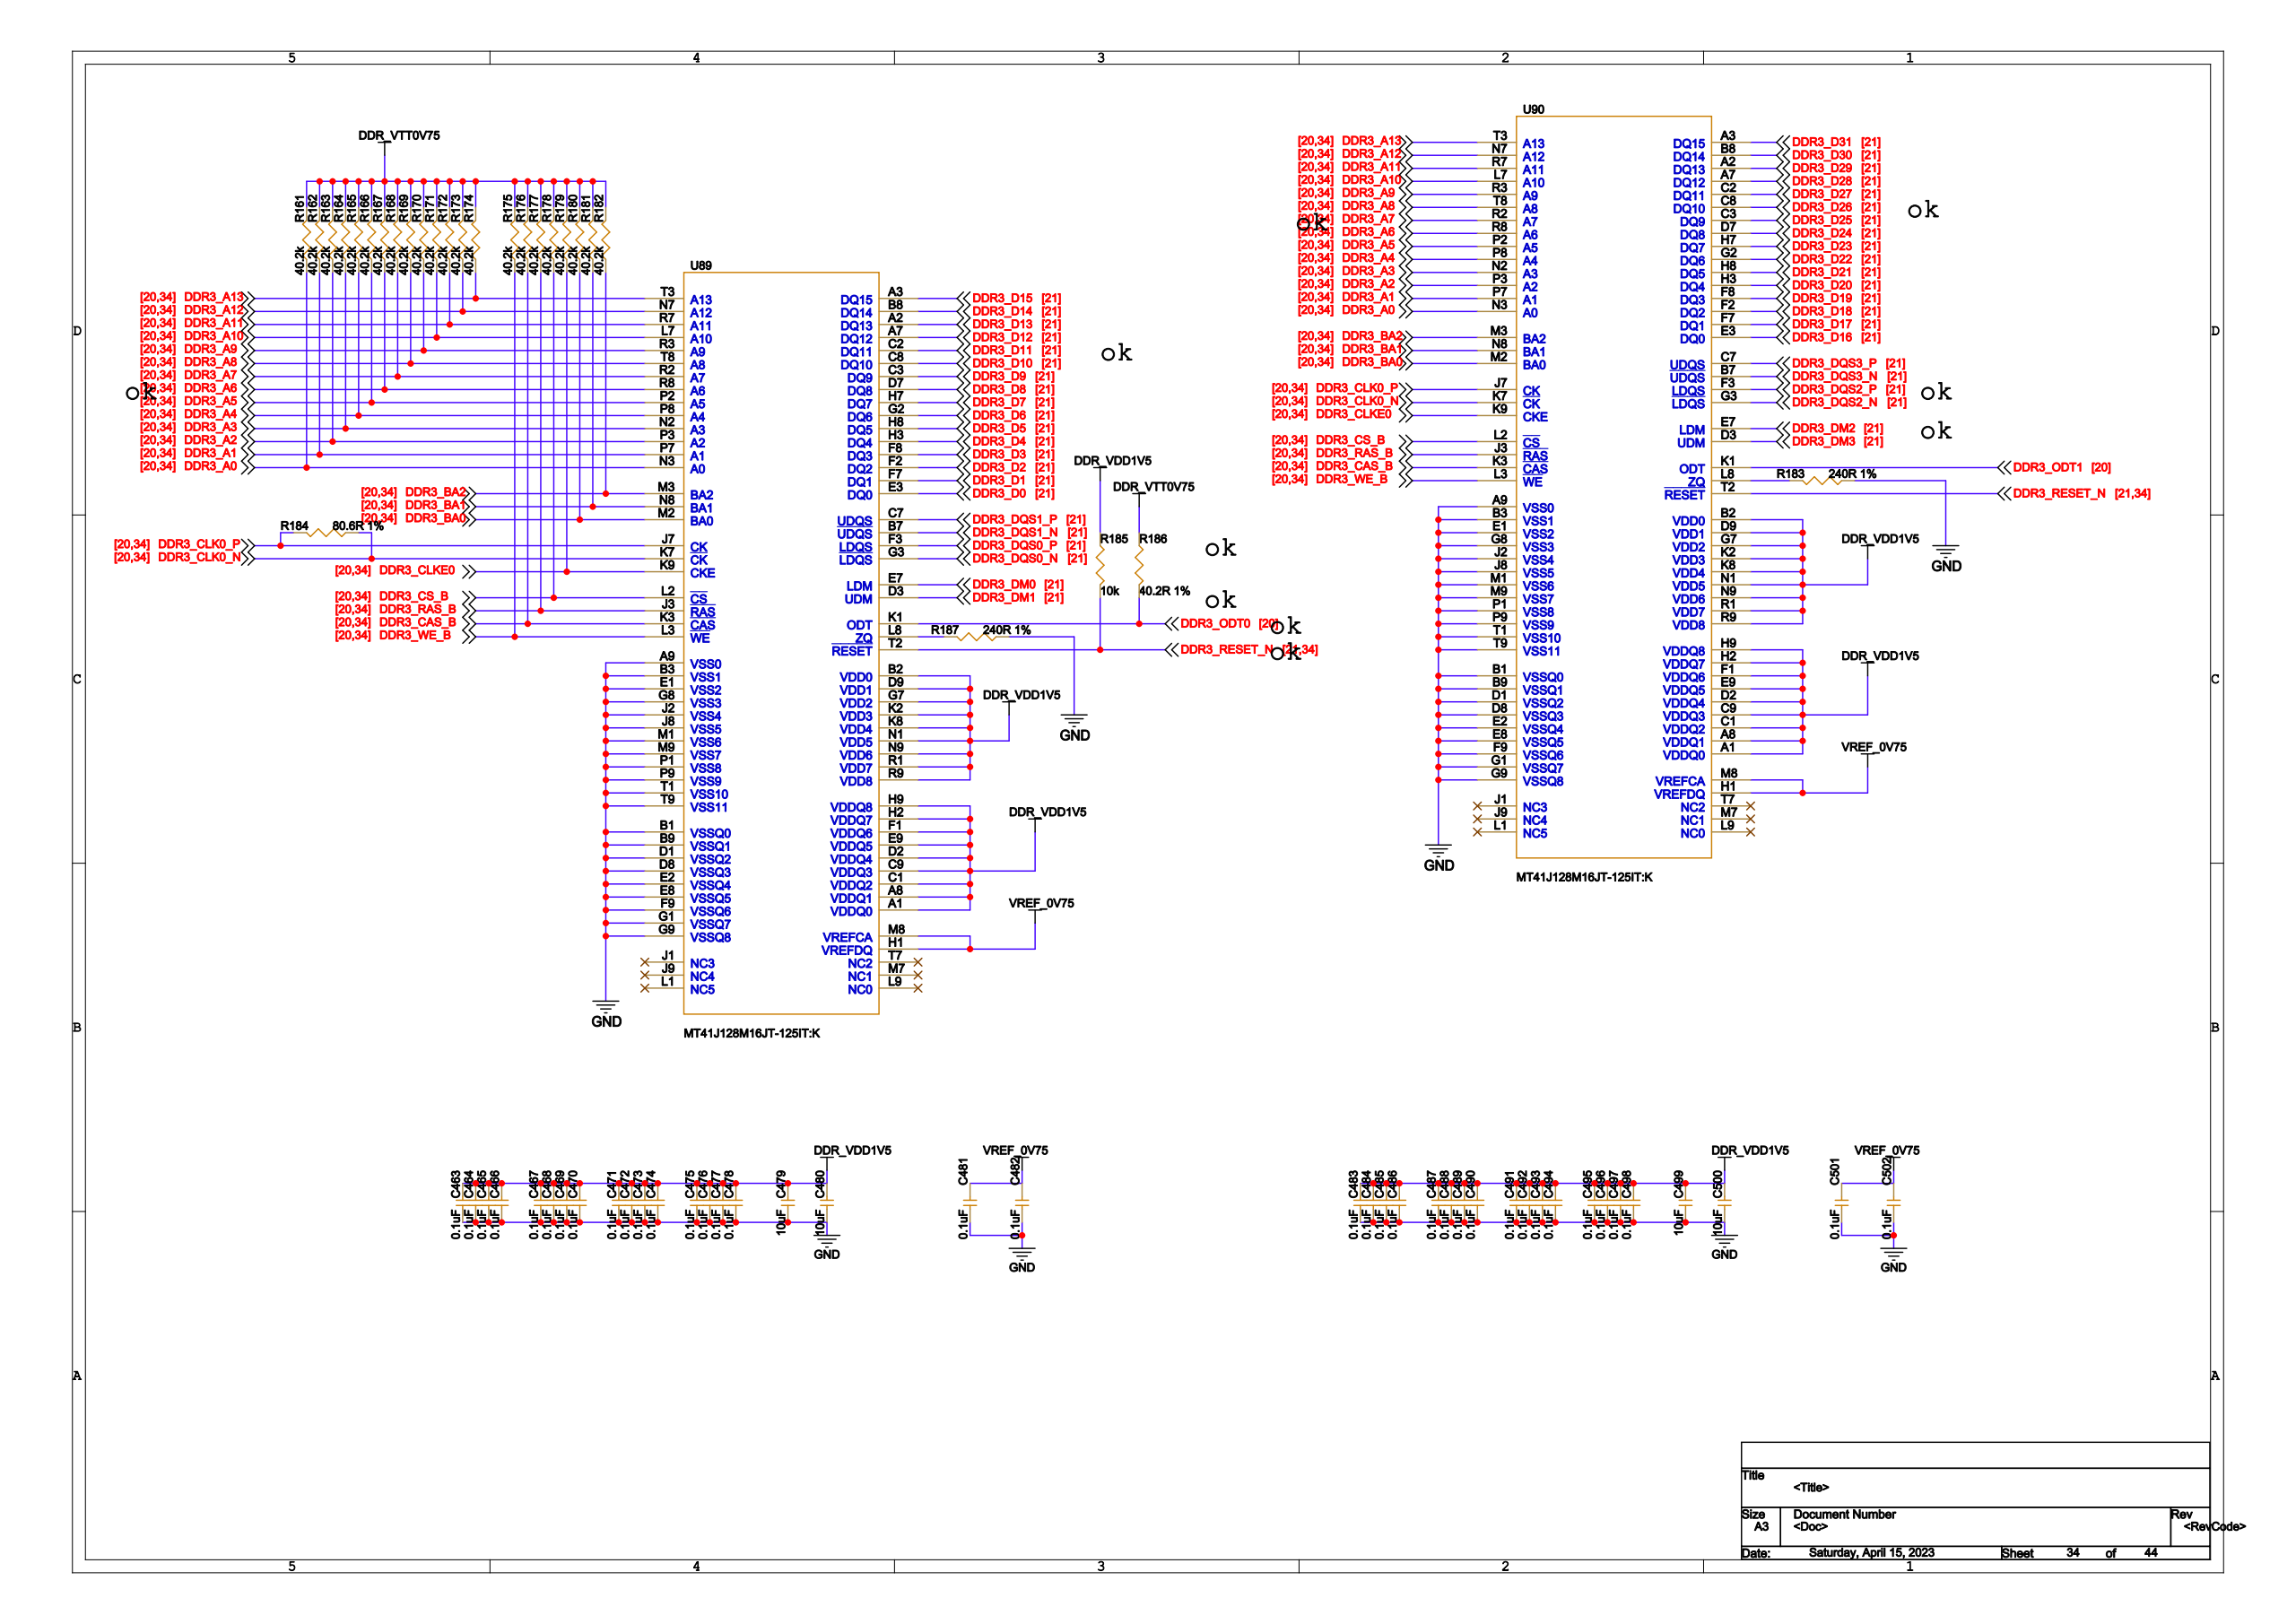Circuit board | Cadence Allegro | 1034 parts | 912 nets | one sheet of the schematic
Parts on this sheet (reference | value | footprint):
C463 | 0.1uF | C0402
C464 | 0.1uF | C0402
C465 | 0.1uF | C0402
C466 | 0.1uF | C0402
C467 | 0.1uF | C0402
C468 | 0.1uF | C0402
C469 | 0.1uF | C0402
C470 | 0.1uF | C0402
C471 | 0.1uF | C0402
C472 | 0.1uF | C0402
C473 | 0.1uF | C0402
C474 | 0.1uF | C0402
C475 | 0.1uF | C0402
C476 | 0.1uF | C0402
C477 | 0.1uF | C0402
C478 | 0.1uF | C0402
C479 | 10uF | C0402
C480 | 10uF | C0402
C481 | 0.1uF | C0402
C482 | 0.1uF | C0402
C483 | 0.1uF | C0402
C484 | 0.1uF | C0402
C485 | 0.1uF | C0402
C486 | 0.1uF | C0402
C487 | 0.1uF | C0402
C488 | 0.1uF | C0402
C489 | 0.1uF | C0402
C490 | 0.1uF | C0402
C491 | 0.1uF | C0402
C492 | 0.1uF | C0402
C493 | 0.1uF | C0402
C494 | 0.1uF | C0402
C495 | 0.1uF | C0402
C496 | 0.1uF | C0402
C497 | 0.1uF | C0402
C498 | 0.1uF | C0402
C499 | 10uF | C0402
C500 | 10uF | C0402
C501 | 0.1uF | C0402
C502 | 0.1uF | C0402
P1 | TSW-120-07-G-D | TSW_2MM54_DR
P3 | TSW-120-07-G-D | TSW_2MM54_DR
R161 | 40.2k | R0402
R162 | 40.2k | R0402
R163 | 40.2k | R0402
R164 | 40.2k | R0402
R165 | 40.2k | R0402
R166 | 40.2k | R0402
R167 | 40.2k | R0402
R168 | 40.2k | R0402
R169 | 40.2k | R0402
R170 | 40.2k | R0402
R171 | 40.2k | R0402
R172 | 40.2k | R0402
R173 | 40.2k | R0402
R174 | 40.2k | R0402
R175 | 40.2k | R0402
R176 | 40.2k | R0402
R177 | 40.2k | R0402
R178 | 40.2k | R0402
R179 | 40.2k | R0402
R180 | 40.2k | R0402
R181 | 40.2k | R0402
R182 | 40.2k | R0402
R183 | 240R 1% | R0402
R184 | 80.6R 1% | R0402
R185 | 10k | R0402
R186 | 40.2R 1% | R0402
R187 | 240R 1% | R0402
U89 | MT41J128M16JT-125IT:K | FBGA_96BALL
U90 | MT41J128M16JT-125IT:K | FBGA_96BALL
Nets of these parts (net: part-pin ...):
GND: C463-1 C464-1 C465-1 C466-1 C467-1 C468-1 C469-1 C470-1 C471-1 C472-1 C473-1 C474-1 C475-1 C476-1 C477-1 C478-1 C479-1 C480-1 C481-1 C482-1 C483-1 C484-1 C485-1 C486-1 C487-1 C488-1 C489-1 C490-1 C491-1 C492-1 C493-1 C494-1 C495-1 C496-1 C497-1 C498-1 C499-1 C500-1 C501-1 C502-1 R183-1 R187-1 P1-1 P1-2 P1-3 P1-4 P1-15 P1-34 P3-1 P3-2 P3-3 P3-15 U89-A9 U89-B1 U89-B3 U89-B9 U89-D1 U89-D8 U89-E1 U89-E2 U89-E8 U89-F9 U89-G1 U89-G8 U89-G9 U89-J2 U89-J8 U89-M1 U89-M9 U89-P1 U89-P9 U89-T1 U89-T9 U90-A9 U90-B1 U90-B3 U90-B9 U90-D1 U90-D8 U90-E1 U90-E2 U90-E8 U90-F9 U90-G1 U90-G8 U90-G9 U90-J2 U90-J8 U90-M1 U90-M9 U90-P1 U90-P9 U90-T1 U90-T9
VREF_0V75: C481-2 C482-2 C501-2 C502-2 U89-H1 U89-M8 U90-H1 U90-M8
DDR3_CLK0_N: R184-1 U89-K7 U90-K7
DDR3_CLK0_P: R184-2 U89-J7 U90-J7
DDR_VTT0V75: R161-2 R162-2 R163-2 R164-2 R165-2 R166-2 R167-2 R168-2 R169-2 R170-2 R171-2 R172-2 R173-2 R174-2 R175-2 R176-2 R177-2 R178-2 R179-2 R180-2 R181-2 R182-2 R186-1
DDR3_ODT0: R186-2 U89-K1
DDR_VDD1V5: C463-2 C464-2 C465-2 C466-2 C467-2 C468-2 C469-2 C470-2 C471-2 C472-2 C473-2 C474-2 C475-2 C476-2 C477-2 C478-2 C479-2 C480-2 C483-2 C484-2 C485-2 C486-2 C487-2 C488-2 C489-2 C490-2 C491-2 C492-2 C493-2 C494-2 C495-2 C496-2 C497-2 C498-2 C499-2 C500-2 R185-1 U89-A1 U89-A8 U89-B2 U89-C1 U89-C9 U89-D2 U89-D9 U89-E9 U89-F1 U89-G7 U89-H2 U89-H9 U89-K2 U89-K8 U89-N1 U89-N9 U89-R1 U89-R9 U90-A1 U90-A8 U90-B2 U90-C1 U90-C9 U90-D2 U90-D9 U90-E9 U90-F1 U90-G7 U90-H2 U90-H9 U90-K2 U90-K8 U90-N1 U90-N9 U90-R1 U90-R9
DDR3_RESET_N: R185-2 U89-T2 U90-T2
DDR3_BA1: R181-1 U89-N8 U90-N8
DDR3_BA2: R182-1 U89-M3 U90-M3
DDR3_A0: R161-1 U89-N3 U90-N3
DDR3_A1: R162-1 U89-P7 U90-P7
DDR3_A2: R163-1 U89-P3 U90-P3
DDR3_A3: R164-1 U89-N2 U90-N2
DDR3_A4: R165-1 U89-P8 U90-P8
DDR3_A5: R166-1 U89-P2 U90-P2
DDR3_A6: R167-1 U89-R8 U90-R8
DDR3_A7: R168-1 U89-R2 U90-R2
DDR3_A8: R169-1 U89-T8 U90-T8
DDR3_A9: R170-1 U89-R3 U90-R3
DDR3_A10: R171-1 U89-L7 U90-L7
DDR3_A11: R172-1 U89-R7 U90-R7
DDR3_A12: R173-1 U89-N7 U90-N7
DDR3_A13: R174-1 U89-T3 U90-T3
DDR3_WE_B: R175-1 U89-L3 U90-L3
DDR3_CAS_B: R176-1 U89-K3 U90-K3
DDR3_RAS_B: R177-1 U89-J3 U90-J3
DDR3_CS_B: R178-1 U89-L2 U90-L2
DDR3_CLKE0: R179-1 U89-K9 U90-K9
DDR3_BA0: R180-1 U89-M2 U90-M2
N13783006: R183-2 U90-L8
N13782287: R187-2 U89-L8
DDR3_ODT1: U90-K1
DDR3_D20: U90-H3
DDR3_D21: U90-H8
DDR3_D18: U90-F2
DDR3_D19: U90-F8
DDR3_D16: U90-E3
DDR3_D17: U90-F7
DDR3_D15: U89-A3
DDR3_D13: U89-A2
DDR3_D14: U89-B8
DDR3_DQS1_N: U89-B7
DDR3_DQS1_P: U89-C7
DDR3_D11: U89-C2
DDR3_D12: U89-A7
DDR3_D9: U89-C3
DDR3_D10: U89-C8
DDR3_DM1: U89-D3
DDR3_D8: U89-D7
DDR3_DM0: U89-E7
DDR3_D30: U90-B8
DDR3_D31: U90-A3
DDR3_D6: U89-G2
DDR3_D7: U89-H7
DDR3_DQS0_N: U89-G3
DDR3_DQS0_P: U89-F3
DDR3_D4: U89-H3
DDR3_D5: U89-H8
DDR3_D2: U89-F2
DDR3_D3: U89-F8
DDR3_D0: U89-E3
DDR3_D1: U89-F7
DDR3_D28: U90-A7
DDR3_D29: U90-A2
DDR3_DQS3_N: U90-B7
DDR3_DQS3_P: U90-C7
DDR3_D26: U90-C8
DDR3_D27: U90-C2
DDR3_D24: U90-D7
DDR3_D25: U90-C3
DDR3_DM2: U90-E7
DDR3_DM3: U90-D3
DDR3_D22: U90-G2
DDR3_D23: U90-H7
DDR3_DQS2_N: U90-G3
DDR3_DQS2_P: U90-F3